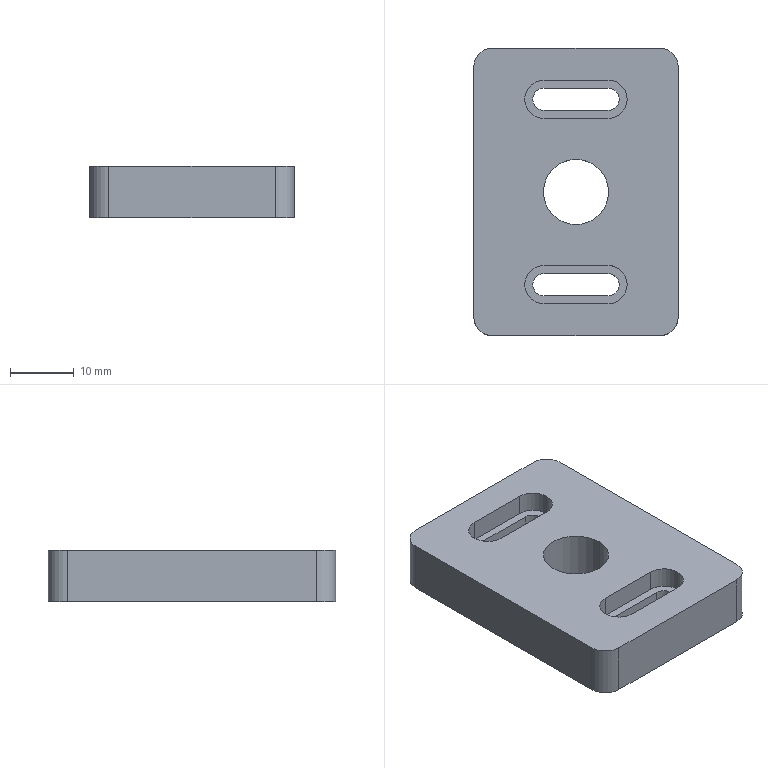Part | SolidWorks | features ICE 2, Extrusion 1, Fillet 1, HoleWzd 1 | 1 solid | 34 faces | box 32 x 45 x 8 mm | volume 9802 mm3 | cylinder 18 | plane 16 | commonest cylinder face diameters 6 x10 3.5 x6 10.2 x2
STEP:
#1=CARTESIAN_POINT('',(8.,14.5,4.7));
#2=VERTEX_POINT('',#1);
#3=CARTESIAN_POINT('',(5.,17.5,4.7));
#4=VERTEX_POINT('',#3);
#5=CARTESIAN_POINT('',(5.,14.5,4.7));
#6=DIRECTION('',(0.,0.,1.));
#7=DIRECTION('',(1.,0.,0.));
#8=AXIS2_PLACEMENT_3D('',#5,#6,#7);
#9=CIRCLE('',#8,3.);
#10=EDGE_CURVE('',#2,#4,#9,.T.);
#11=ORIENTED_EDGE('',*,*,#10,.F.);
#12=CARTESIAN_POINT('',(8.,14.5,8.));
#13=VERTEX_POINT('',#12);
#14=CARTESIAN_POINT('',(8.,14.5,4.7));
#15=DIRECTION('',(0.,0.,1.));
#16=VECTOR('',#15,1000.);
#17=LINE('',#14,#16);
#18=EDGE_CURVE('',#2,#13,#17,.T.);
#19=ORIENTED_EDGE('',*,*,#18,.T.);
#20=CARTESIAN_POINT('',(5.,17.5,8.));
#21=VERTEX_POINT('',#20);
#22=CARTESIAN_POINT('',(5.,14.5,8.));
#23=DIRECTION('',(0.,0.,1.));
#24=DIRECTION('',(1.,0.,0.));
#25=AXIS2_PLACEMENT_3D('',#22,#23,#24);
#26=CIRCLE('',#25,3.);
#27=EDGE_CURVE('',#13,#21,#26,.T.);
#28=ORIENTED_EDGE('',*,*,#27,.T.);
#29=CARTESIAN_POINT('',(5.,17.5,4.7));
#30=DIRECTION('',(0.,0.,1.));
#31=VECTOR('',#30,1000.);
#32=LINE('',#29,#31);
#33=EDGE_CURVE('',#4,#21,#32,.T.);
#34=ORIENTED_EDGE('',*,*,#33,.F.);
#35=EDGE_LOOP('',(#11,#19,#28,#34));
#36=FACE_OUTER_BOUND('',#35,.T.);
#37=CARTESIAN_POINT('',(5.,14.5,4.7));
#38=DIRECTION('',(0.,0.,1.));
#39=DIRECTION('',(1.,0.,0.));
#40=AXIS2_PLACEMENT_3D('',#37,#38,#39);
#41=CYLINDRICAL_SURFACE('',#40,3.);
#42=ADVANCED_FACE('',(#36),#41,.F.);
#43=CARTESIAN_POINT('',(8.,-14.5,4.7));
#44=VERTEX_POINT('',#43);
#45=CARTESIAN_POINT('',(5.,-11.5,4.7));
#46=VERTEX_POINT('',#45);
#47=CARTESIAN_POINT('',(5.,-14.5,4.7));
#48=DIRECTION('',(0.,0.,1.));
#49=DIRECTION('',(1.,0.,0.));
#50=AXIS2_PLACEMENT_3D('',#47,#48,#49);
#51=CIRCLE('',#50,3.);
#52=EDGE_CURVE('',#44,#46,#51,.T.);
#53=ORIENTED_EDGE('',*,*,#52,.F.);
#54=CARTESIAN_POINT('',(8.,-14.5,8.));
#55=VERTEX_POINT('',#54);
#56=CARTESIAN_POINT('',(8.,-14.5,4.7));
#57=DIRECTION('',(0.,0.,1.));
#58=VECTOR('',#57,1000.);
#59=LINE('',#56,#58);
#60=EDGE_CURVE('',#44,#55,#59,.T.);
#61=ORIENTED_EDGE('',*,*,#60,.T.);
#62=CARTESIAN_POINT('',(5.,-11.5,8.));
#63=VERTEX_POINT('',#62);
#64=CARTESIAN_POINT('',(5.,-14.5,8.));
#65=DIRECTION('',(0.,0.,1.));
#66=DIRECTION('',(1.,0.,0.));
#67=AXIS2_PLACEMENT_3D('',#64,#65,#66);
#68=CIRCLE('',#67,3.);
#69=EDGE_CURVE('',#55,#63,#68,.T.);
#70=ORIENTED_EDGE('',*,*,#69,.T.);
#71=CARTESIAN_POINT('',(5.,-11.5,4.7));
#72=DIRECTION('',(0.,0.,1.));
#73=VECTOR('',#72,1000.);
#74=LINE('',#71,#73);
#75=EDGE_CURVE('',#46,#63,#74,.T.);
#76=ORIENTED_EDGE('',*,*,#75,.F.);
#77=EDGE_LOOP('',(#53,#61,#70,#76));
#78=FACE_OUTER_BOUND('',#77,.T.);
#79=CARTESIAN_POINT('',(5.,-14.5,4.7));
#80=DIRECTION('',(0.,0.,1.));
#81=DIRECTION('',(1.,0.,0.));
#82=AXIS2_PLACEMENT_3D('',#79,#80,#81);
#83=CYLINDRICAL_SURFACE('',#82,3.);
#84=ADVANCED_FACE('',(#78),#83,.F.);
#85=CARTESIAN_POINT('',(-5.1,0.,0.));
#86=VERTEX_POINT('',#85);
#87=CARTESIAN_POINT('',(5.1,0.,0.));
#88=VERTEX_POINT('',#87);
#89=CARTESIAN_POINT('',(0.,0.,0.));
#90=DIRECTION('',(0.,0.,1.));
#91=DIRECTION('',(1.,0.,0.));
#92=AXIS2_PLACEMENT_3D('',#89,#90,#91);
#93=CIRCLE('',#92,5.1);
#94=EDGE_CURVE('',#86,#88,#93,.T.);
#95=ORIENTED_EDGE('',*,*,#94,.F.);
#96=CARTESIAN_POINT('',(-5.1,0.,8.));
#97=VERTEX_POINT('',#96);
#98=CARTESIAN_POINT('',(-5.1,0.,8.));
#99=DIRECTION('',(0.,0.,1.));
#100=VECTOR('',#99,1000.);
#101=LINE('',#98,#100);
#102=EDGE_CURVE('',#86,#97,#101,.T.);
#103=ORIENTED_EDGE('',*,*,#102,.T.);
#104=CARTESIAN_POINT('',(5.1,0.,8.));
#105=VERTEX_POINT('',#104);
#106=CARTESIAN_POINT('',(0.,0.,8.));
#107=DIRECTION('',(0.,0.,1.));
#108=DIRECTION('',(1.,0.,0.));
#109=AXIS2_PLACEMENT_3D('',#106,#107,#108);
#110=CIRCLE('',#109,5.1);
#111=EDGE_CURVE('',#97,#105,#110,.T.);
#112=ORIENTED_EDGE('',*,*,#111,.T.);
#113=CARTESIAN_POINT('',(5.1,0.,8.));
#114=DIRECTION('',(0.,0.,1.));
#115=VECTOR('',#114,1000.);
#116=LINE('',#113,#115);
#117=EDGE_CURVE('',#88,#105,#116,.T.);
#118=ORIENTED_EDGE('',*,*,#117,.F.);
#119=EDGE_LOOP('',(#95,#103,#112,#118));
#120=FACE_OUTER_BOUND('',#119,.T.);
#121=CARTESIAN_POINT('',(0.,0.,8.));
#122=DIRECTION('',(0.,0.,1.));
#123=DIRECTION('',(1.,0.,0.));
#124=AXIS2_PLACEMENT_3D('',#121,#122,#123);
#125=CYLINDRICAL_SURFACE('',#124,5.1);
#126=ADVANCED_FACE('',(#120),#125,.F.);
#127=CARTESIAN_POINT('',(6.75,-14.5,0.));
#128=VERTEX_POINT('',#127);
#129=CARTESIAN_POINT('',(5.,-12.75,0.));
#130=VERTEX_POINT('',#129);
#131=CARTESIAN_POINT('',(5.,-14.5,0.));
#132=DIRECTION('',(0.,0.,1.));
#133=DIRECTION('',(1.,0.,0.));
#134=AXIS2_PLACEMENT_3D('',#131,#132,#133);
#135=CIRCLE('',#134,1.75);
#136=EDGE_CURVE('',#128,#130,#135,.T.);
#137=ORIENTED_EDGE('',*,*,#136,.F.);
#138=CARTESIAN_POINT('',(6.75,-14.5,4.7));
#139=VERTEX_POINT('',#138);
#140=CARTESIAN_POINT('',(6.75,-14.5,0.));
#141=DIRECTION('',(0.,0.,1.));
#142=VECTOR('',#141,1000.);
#143=LINE('',#140,#142);
#144=EDGE_CURVE('',#128,#139,#143,.T.);
#145=ORIENTED_EDGE('',*,*,#144,.T.);
#146=CARTESIAN_POINT('',(5.,-12.75,4.7));
#147=VERTEX_POINT('',#146);
#148=CARTESIAN_POINT('',(5.,-14.5,4.7));
#149=DIRECTION('',(0.,0.,-1.));
#150=DIRECTION('',(1.,0.,0.));
#151=AXIS2_PLACEMENT_3D('',#148,#149,#150);
#152=CIRCLE('',#151,1.75);
#153=EDGE_CURVE('',#147,#139,#152,.T.);
#154=ORIENTED_EDGE('',*,*,#153,.F.);
#155=CARTESIAN_POINT('',(5.,-12.75,0.));
#156=DIRECTION('',(0.,0.,1.));
#157=VECTOR('',#156,1000.);
#158=LINE('',#155,#157);
#159=EDGE_CURVE('',#130,#147,#158,.T.);
#160=ORIENTED_EDGE('',*,*,#159,.F.);
#161=EDGE_LOOP('',(#137,#145,#154,#160));
#162=FACE_OUTER_BOUND('',#161,.T.);
#163=CARTESIAN_POINT('',(5.,-14.5,0.));
#164=DIRECTION('',(0.,0.,1.));
#165=DIRECTION('',(1.,0.,0.));
#166=AXIS2_PLACEMENT_3D('',#163,#164,#165);
#167=CYLINDRICAL_SURFACE('',#166,1.75);
#168=ADVANCED_FACE('',(#162),#167,.F.);
#169=CARTESIAN_POINT('',(6.75,14.5,0.));
#170=VERTEX_POINT('',#169);
#171=CARTESIAN_POINT('',(5.,16.25,0.));
#172=VERTEX_POINT('',#171);
#173=CARTESIAN_POINT('',(5.,14.5,0.));
#174=DIRECTION('',(0.,0.,1.));
#175=DIRECTION('',(1.,0.,0.));
#176=AXIS2_PLACEMENT_3D('',#173,#174,#175);
#177=CIRCLE('',#176,1.75);
#178=EDGE_CURVE('',#170,#172,#177,.T.);
#179=ORIENTED_EDGE('',*,*,#178,.F.);
#180=CARTESIAN_POINT('',(6.75,14.5,4.7));
#181=VERTEX_POINT('',#180);
#182=CARTESIAN_POINT('',(6.75,14.5,0.));
#183=DIRECTION('',(0.,0.,1.));
#184=VECTOR('',#183,1000.);
#185=LINE('',#182,#184);
#186=EDGE_CURVE('',#170,#181,#185,.T.);
#187=ORIENTED_EDGE('',*,*,#186,.T.);
#188=CARTESIAN_POINT('',(5.,16.25,4.7));
#189=VERTEX_POINT('',#188);
#190=CARTESIAN_POINT('',(5.,14.5,4.7));
#191=DIRECTION('',(0.,0.,-1.));
#192=DIRECTION('',(1.,0.,0.));
#193=AXIS2_PLACEMENT_3D('',#190,#191,#192);
#194=CIRCLE('',#193,1.75);
#195=EDGE_CURVE('',#189,#181,#194,.T.);
#196=ORIENTED_EDGE('',*,*,#195,.F.);
#197=CARTESIAN_POINT('',(5.,16.25,0.));
#198=DIRECTION('',(0.,0.,1.));
#199=VECTOR('',#198,1000.);
#200=LINE('',#197,#199);
#201=EDGE_CURVE('',#172,#189,#200,.T.);
#202=ORIENTED_EDGE('',*,*,#201,.F.);
#203=EDGE_LOOP('',(#179,#187,#196,#202));
#204=FACE_OUTER_BOUND('',#203,.T.);
#205=CARTESIAN_POINT('',(5.,14.5,0.));
#206=DIRECTION('',(0.,0.,1.));
#207=DIRECTION('',(1.,0.,0.));
#208=AXIS2_PLACEMENT_3D('',#205,#206,#207);
#209=CYLINDRICAL_SURFACE('',#208,1.75);
#210=ADVANCED_FACE('',(#204),#209,.F.);
#211=CARTESIAN_POINT('',(-5.,12.75,4.7));
#212=VERTEX_POINT('',#211);
#213=CARTESIAN_POINT('',(-5.,16.25,4.7));
#214=VERTEX_POINT('',#213);
#215=CARTESIAN_POINT('',(-5.,14.5,4.7));
#216=DIRECTION('',(0.,0.,-1.));
#217=DIRECTION('',(1.,0.,0.));
#218=AXIS2_PLACEMENT_3D('',#215,#216,#217);
#219=CIRCLE('',#218,1.75);
#220=EDGE_CURVE('',#212,#214,#219,.T.);
#221=ORIENTED_EDGE('',*,*,#220,.F.);
#222=CARTESIAN_POINT('',(-5.,12.75,0.));
#223=VERTEX_POINT('',#222);
#224=CARTESIAN_POINT('',(-5.,12.75,0.));
#225=DIRECTION('',(0.,0.,1.));
#226=VECTOR('',#225,1000.);
#227=LINE('',#224,#226);
#228=EDGE_CURVE('',#223,#212,#227,.T.);
#229=ORIENTED_EDGE('',*,*,#228,.F.);
#230=CARTESIAN_POINT('',(-5.,16.25,0.));
#231=VERTEX_POINT('',#230);
#232=CARTESIAN_POINT('',(-5.,14.5,0.));
#233=DIRECTION('',(0.,0.,1.));
#234=DIRECTION('',(1.,0.,0.));
#235=AXIS2_PLACEMENT_3D('',#232,#233,#234);
#236=CIRCLE('',#235,1.75);
#237=EDGE_CURVE('',#231,#223,#236,.T.);
#238=ORIENTED_EDGE('',*,*,#237,.F.);
#239=CARTESIAN_POINT('',(-5.,16.25,0.));
#240=DIRECTION('',(0.,0.,1.));
#241=VECTOR('',#240,1000.);
#242=LINE('',#239,#241);
#243=EDGE_CURVE('',#231,#214,#242,.T.);
#244=ORIENTED_EDGE('',*,*,#243,.T.);
#245=EDGE_LOOP('',(#221,#229,#238,#244));
#246=FACE_OUTER_BOUND('',#245,.T.);
#247=CARTESIAN_POINT('',(-5.,14.5,0.));
#248=DIRECTION('',(0.,0.,1.));
#249=DIRECTION('',(1.,0.,0.));
#250=AXIS2_PLACEMENT_3D('',#247,#248,#249);
#251=CYLINDRICAL_SURFACE('',#250,1.75);
#252=ADVANCED_FACE('',(#246),#251,.F.);
#253=CARTESIAN_POINT('',(-5.,16.25,4.7));
#254=DIRECTION('',(1.,0.,0.));
#255=VECTOR('',#254,1000.);
#256=LINE('',#253,#255);
#257=EDGE_CURVE('',#214,#189,#256,.T.);
#258=ORIENTED_EDGE('',*,*,#257,.F.);
#259=ORIENTED_EDGE('',*,*,#243,.F.);
#260=CARTESIAN_POINT('',(-5.,16.25,0.));
#261=DIRECTION('',(-1.,0.,0.));
#262=VECTOR('',#261,1000.);
#263=LINE('',#260,#262);
#264=EDGE_CURVE('',#172,#231,#263,.T.);
#265=ORIENTED_EDGE('',*,*,#264,.F.);
#266=ORIENTED_EDGE('',*,*,#201,.T.);
#267=EDGE_LOOP('',(#258,#259,#265,#266));
#268=FACE_OUTER_BOUND('',#267,.T.);
#269=CARTESIAN_POINT('',(-5.,16.25,0.));
#270=DIRECTION('',(0.,1.,0.));
#271=DIRECTION('',(-1.,0.,0.));
#272=AXIS2_PLACEMENT_3D('',#269,#270,#271);
#273=PLANE('',#272);
#274=ADVANCED_FACE('',(#268),#273,.F.);
#275=ORIENTED_EDGE('',*,*,#186,.F.);
#276=CARTESIAN_POINT('',(5.,12.75,0.));
#277=VERTEX_POINT('',#276);
#278=CARTESIAN_POINT('',(5.,14.5,0.));
#279=DIRECTION('',(0.,0.,1.));
#280=DIRECTION('',(1.,0.,0.));
#281=AXIS2_PLACEMENT_3D('',#278,#279,#280);
#282=CIRCLE('',#281,1.75);
#283=EDGE_CURVE('',#277,#170,#282,.T.);
#284=ORIENTED_EDGE('',*,*,#283,.F.);
#285=CARTESIAN_POINT('',(5.,12.75,4.7));
#286=VERTEX_POINT('',#285);
#287=CARTESIAN_POINT('',(5.,12.75,0.));
#288=DIRECTION('',(0.,0.,1.));
#289=VECTOR('',#288,1000.);
#290=LINE('',#287,#289);
#291=EDGE_CURVE('',#277,#286,#290,.T.);
#292=ORIENTED_EDGE('',*,*,#291,.T.);
#293=CARTESIAN_POINT('',(5.,14.5,4.7));
#294=DIRECTION('',(0.,0.,-1.));
#295=DIRECTION('',(1.,0.,0.));
#296=AXIS2_PLACEMENT_3D('',#293,#294,#295);
#297=CIRCLE('',#296,1.75);
#298=EDGE_CURVE('',#181,#286,#297,.T.);
#299=ORIENTED_EDGE('',*,*,#298,.F.);
#300=EDGE_LOOP('',(#275,#284,#292,#299));
#301=FACE_OUTER_BOUND('',#300,.T.);
#302=CARTESIAN_POINT('',(5.,14.5,0.));
#303=DIRECTION('',(0.,0.,1.));
#304=DIRECTION('',(1.,0.,0.));
#305=AXIS2_PLACEMENT_3D('',#302,#303,#304);
#306=CYLINDRICAL_SURFACE('',#305,1.75);
#307=ADVANCED_FACE('',(#301),#306,.F.);
#308=CARTESIAN_POINT('',(-5.,12.75,4.7));
#309=DIRECTION('',(-1.,0.,0.));
#310=VECTOR('',#309,1000.);
#311=LINE('',#308,#310);
#312=EDGE_CURVE('',#286,#212,#311,.T.);
#313=ORIENTED_EDGE('',*,*,#312,.F.);
#314=ORIENTED_EDGE('',*,*,#291,.F.);
#315=CARTESIAN_POINT('',(-5.,12.75,0.));
#316=DIRECTION('',(1.,0.,0.));
#317=VECTOR('',#316,1000.);
#318=LINE('',#315,#317);
#319=EDGE_CURVE('',#223,#277,#318,.T.);
#320=ORIENTED_EDGE('',*,*,#319,.F.);
#321=ORIENTED_EDGE('',*,*,#228,.T.);
#322=EDGE_LOOP('',(#313,#314,#320,#321));
#323=FACE_OUTER_BOUND('',#322,.T.);
#324=CARTESIAN_POINT('',(-5.,12.75,0.));
#325=DIRECTION('',(0.,-1.,0.));
#326=DIRECTION('',(0.,0.,-1.));
#327=AXIS2_PLACEMENT_3D('',#324,#325,#326);
#328=PLANE('',#327);
#329=ADVANCED_FACE('',(#323),#328,.F.);
#330=CARTESIAN_POINT('',(-5.,-16.25,4.7));
#331=VERTEX_POINT('',#330);
#332=CARTESIAN_POINT('',(-5.,-12.75,4.7));
#333=VERTEX_POINT('',#332);
#334=CARTESIAN_POINT('',(-5.,-14.5,4.7));
#335=DIRECTION('',(0.,0.,-1.));
#336=DIRECTION('',(1.,0.,0.));
#337=AXIS2_PLACEMENT_3D('',#334,#335,#336);
#338=CIRCLE('',#337,1.75);
#339=EDGE_CURVE('',#331,#333,#338,.T.);
#340=ORIENTED_EDGE('',*,*,#339,.F.);
#341=CARTESIAN_POINT('',(-5.,-16.25,0.));
#342=VERTEX_POINT('',#341);
#343=CARTESIAN_POINT('',(-5.,-16.25,0.));
#344=DIRECTION('',(0.,0.,1.));
#345=VECTOR('',#344,1000.);
#346=LINE('',#343,#345);
#347=EDGE_CURVE('',#342,#331,#346,.T.);
#348=ORIENTED_EDGE('',*,*,#347,.F.);
#349=CARTESIAN_POINT('',(-5.,-12.75,0.));
#350=VERTEX_POINT('',#349);
#351=CARTESIAN_POINT('',(-5.,-14.5,0.));
#352=DIRECTION('',(0.,0.,1.));
#353=DIRECTION('',(1.,0.,0.));
#354=AXIS2_PLACEMENT_3D('',#351,#352,#353);
#355=CIRCLE('',#354,1.75);
#356=EDGE_CURVE('',#350,#342,#355,.T.);
#357=ORIENTED_EDGE('',*,*,#356,.F.);
#358=CARTESIAN_POINT('',(-5.,-12.75,0.));
#359=DIRECTION('',(0.,0.,1.));
#360=VECTOR('',#359,1000.);
#361=LINE('',#358,#360);
#362=EDGE_CURVE('',#350,#333,#361,.T.);
#363=ORIENTED_EDGE('',*,*,#362,.T.);
#364=EDGE_LOOP('',(#340,#348,#357,#363));
#365=FACE_OUTER_BOUND('',#364,.T.);
#366=CARTESIAN_POINT('',(-5.,-14.5,0.));
#367=DIRECTION('',(0.,0.,1.));
#368=DIRECTION('',(1.,0.,0.));
#369=AXIS2_PLACEMENT_3D('',#366,#367,#368);
#370=CYLINDRICAL_SURFACE('',#369,1.75);
#371=ADVANCED_FACE('',(#365),#370,.F.);
#372=CARTESIAN_POINT('',(-5.,-12.75,4.7));
#373=DIRECTION('',(1.,0.,0.));
#374=VECTOR('',#373,1000.);
#375=LINE('',#372,#374);
#376=EDGE_CURVE('',#333,#147,#375,.T.);
#377=ORIENTED_EDGE('',*,*,#376,.F.);
#378=ORIENTED_EDGE('',*,*,#362,.F.);
#379=CARTESIAN_POINT('',(-5.,-12.75,0.));
#380=DIRECTION('',(-1.,0.,0.));
#381=VECTOR('',#380,1000.);
#382=LINE('',#379,#381);
#383=EDGE_CURVE('',#130,#350,#382,.T.);
#384=ORIENTED_EDGE('',*,*,#383,.F.);
#385=ORIENTED_EDGE('',*,*,#159,.T.);
#386=EDGE_LOOP('',(#377,#378,#384,#385));
#387=FACE_OUTER_BOUND('',#386,.T.);
#388=CARTESIAN_POINT('',(-5.,-12.75,0.));
#389=DIRECTION('',(0.,1.,0.));
#390=DIRECTION('',(0.,0.,1.));
#391=AXIS2_PLACEMENT_3D('',#388,#389,#390);
#392=PLANE('',#391);
#393=ADVANCED_FACE('',(#387),#392,.F.);
#394=ORIENTED_EDGE('',*,*,#144,.F.);
#395=CARTESIAN_POINT('',(5.,-16.25,0.));
#396=VERTEX_POINT('',#395);
#397=CARTESIAN_POINT('',(5.,-14.5,0.));
#398=DIRECTION('',(0.,0.,1.));
#399=DIRECTION('',(1.,0.,0.));
#400=AXIS2_PLACEMENT_3D('',#397,#398,#399);
#401=CIRCLE('',#400,1.75);
#402=EDGE_CURVE('',#396,#128,#401,.T.);
#403=ORIENTED_EDGE('',*,*,#402,.F.);
#404=CARTESIAN_POINT('',(5.,-16.25,4.7));
#405=VERTEX_POINT('',#404);
#406=CARTESIAN_POINT('',(5.,-16.25,0.));
#407=DIRECTION('',(0.,0.,1.));
#408=VECTOR('',#407,1000.);
#409=LINE('',#406,#408);
#410=EDGE_CURVE('',#396,#405,#409,.T.);
#411=ORIENTED_EDGE('',*,*,#410,.T.);
#412=CARTESIAN_POINT('',(5.,-14.5,4.7));
#413=DIRECTION('',(0.,0.,-1.));
#414=DIRECTION('',(1.,0.,0.));
#415=AXIS2_PLACEMENT_3D('',#412,#413,#414);
#416=CIRCLE('',#415,1.75);
#417=EDGE_CURVE('',#139,#405,#416,.T.);
#418=ORIENTED_EDGE('',*,*,#417,.F.);
#419=EDGE_LOOP('',(#394,#403,#411,#418));
#420=FACE_OUTER_BOUND('',#419,.T.);
#421=CARTESIAN_POINT('',(5.,-14.5,0.));
#422=DIRECTION('',(0.,0.,1.));
#423=DIRECTION('',(1.,0.,0.));
#424=AXIS2_PLACEMENT_3D('',#421,#422,#423);
#425=CYLINDRICAL_SURFACE('',#424,1.75);
#426=ADVANCED_FACE('',(#420),#425,.F.);
#427=CARTESIAN_POINT('',(-5.,-16.25,4.7));
#428=DIRECTION('',(-1.,0.,0.));
#429=VECTOR('',#428,1000.);
#430=LINE('',#427,#429);
#431=EDGE_CURVE('',#405,#331,#430,.T.);
#432=ORIENTED_EDGE('',*,*,#431,.F.);
#433=ORIENTED_EDGE('',*,*,#410,.F.);
#434=CARTESIAN_POINT('',(-5.,-16.25,0.));
#435=DIRECTION('',(1.,0.,0.));
#436=VECTOR('',#435,1000.);
#437=LINE('',#434,#436);
#438=EDGE_CURVE('',#342,#396,#437,.T.);
#439=ORIENTED_EDGE('',*,*,#438,.F.);
#440=ORIENTED_EDGE('',*,*,#347,.T.);
#441=EDGE_LOOP('',(#432,#433,#439,#440));
#442=FACE_OUTER_BOUND('',#441,.T.);
#443=CARTESIAN_POINT('',(-5.,-16.25,0.));
#444=DIRECTION('',(0.,-1.,0.));
#445=DIRECTION('',(1.,0.,0.));
#446=AXIS2_PLACEMENT_3D('',#443,#444,#445);
#447=PLANE('',#446);
#448=ADVANCED_FACE('',(#442),#447,.F.);
#449=CARTESIAN_POINT('',(-16.,19.5,8.));
#450=VERTEX_POINT('',#449);
#451=CARTESIAN_POINT('',(-16.,-19.5,8.));
#452=VERTEX_POINT('',#451);
#453=CARTESIAN_POINT('',(-16.,-22.5,8.));
#454=DIRECTION('',(0.,-1.,0.));
#455=VECTOR('',#454,1000.);
#456=LINE('',#453,#455);
#457=EDGE_CURVE('',#450,#452,#456,.T.);
#458=ORIENTED_EDGE('',*,*,#457,.F.);
#459=CARTESIAN_POINT('',(-16.,19.5,0.));
#460=VERTEX_POINT('',#459);
#461=CARTESIAN_POINT('',(-16.,19.5,8.));
#462=DIRECTION('',(0.,0.,-1.));
#463=VECTOR('',#462,1000.);
#464=LINE('',#461,#463);
#465=EDGE_CURVE('',#450,#460,#464,.T.);
#466=ORIENTED_EDGE('',*,*,#465,.T.);
#467=CARTESIAN_POINT('',(-16.,-19.5,0.));
#468=VERTEX_POINT('',#467);
#469=CARTESIAN_POINT('',(-16.,-22.5,0.));
#470=DIRECTION('',(0.,-1.,0.));
#471=VECTOR('',#470,1000.);
#472=LINE('',#469,#471);
#473=EDGE_CURVE('',#460,#468,#472,.T.);
#474=ORIENTED_EDGE('',*,*,#473,.T.);
#475=CARTESIAN_POINT('',(-16.,-19.5,8.));
#476=DIRECTION('',(0.,0.,1.));
#477=VECTOR('',#476,1000.);
#478=LINE('',#475,#477);
#479=EDGE_CURVE('',#468,#452,#478,.T.);
#480=ORIENTED_EDGE('',*,*,#479,.T.);
#481=EDGE_LOOP('',(#458,#466,#474,#480));
#482=FACE_OUTER_BOUND('',#481,.T.);
#483=CARTESIAN_POINT('',(-16.,-22.5,8.));
#484=DIRECTION('',(1.,0.,0.));
#485=DIRECTION('',(0.,0.,-1.));
#486=AXIS2_PLACEMENT_3D('',#483,#484,#485);
#487=PLANE('',#486);
#488=ADVANCED_FACE('',(#482),#487,.F.);
#489=CARTESIAN_POINT('',(-13.,-22.5,0.));
#490=VERTEX_POINT('',#489);
#491=CARTESIAN_POINT('',(13.,-22.5,0.));
#492=VERTEX_POINT('',#491);
#493=CARTESIAN_POINT('',(16.,-22.5,0.));
#494=DIRECTION('',(1.,0.,0.));
#495=VECTOR('',#494,1000.);
#496=LINE('',#493,#495);
#497=EDGE_CURVE('',#490,#492,#496,.T.);
#498=ORIENTED_EDGE('',*,*,#497,.T.);
#499=CARTESIAN_POINT('',(13.,-22.5,8.));
#500=VERTEX_POINT('',#499);
#501=CARTESIAN_POINT('',(13.,-22.5,8.));
#502=DIRECTION('',(0.,0.,1.));
#503=VECTOR('',#502,1000.);
#504=LINE('',#501,#503);
#505=EDGE_CURVE('',#492,#500,#504,.T.);
#506=ORIENTED_EDGE('',*,*,#505,.T.);
#507=CARTESIAN_POINT('',(-13.,-22.5,8.));
#508=VERTEX_POINT('',#507);
#509=CARTESIAN_POINT('',(16.,-22.5,8.));
#510=DIRECTION('',(1.,0.,0.));
#511=VECTOR('',#510,1000.);
#512=LINE('',#509,#511);
#513=EDGE_CURVE('',#508,#500,#512,.T.);
#514=ORIENTED_EDGE('',*,*,#513,.F.);
#515=CARTESIAN_POINT('',(-13.,-22.5,8.));
#516=DIRECTION('',(0.,0.,-1.));
#517=VECTOR('',#516,1000.);
#518=LINE('',#515,#517);
#519=EDGE_CURVE('',#508,#490,#518,.T.);
#520=ORIENTED_EDGE('',*,*,#519,.T.);
#521=EDGE_LOOP('',(#498,#506,#514,#520));
#522=FACE_OUTER_BOUND('',#521,.T.);
#523=CARTESIAN_POINT('',(16.,-22.5,8.));
#524=DIRECTION('',(0.,1.,0.));
#525=DIRECTION('',(-1.,0.,0.));
#526=AXIS2_PLACEMENT_3D('',#523,#524,#525);
#527=PLANE('',#526);
#528=ADVANCED_FACE('',(#522),#527,.F.);
#529=CARTESIAN_POINT('',(16.,-19.5,0.));
#530=VERTEX_POINT('',#529);
#531=CARTESIAN_POINT('',(16.,19.5,0.));
#532=VERTEX_POINT('',#531);
#533=CARTESIAN_POINT('',(16.,-22.5,0.));
#534=DIRECTION('',(0.,1.,0.));
#535=VECTOR('',#534,1000.);
#536=LINE('',#533,#535);
#537=EDGE_CURVE('',#530,#532,#536,.T.);
#538=ORIENTED_EDGE('',*,*,#537,.T.);
#539=CARTESIAN_POINT('',(16.,19.5,8.));
#540=VERTEX_POINT('',#539);
#541=CARTESIAN_POINT('',(16.,19.5,8.));
#542=DIRECTION('',(0.,0.,1.));
#543=VECTOR('',#542,1000.);
#544=LINE('',#541,#543);
#545=EDGE_CURVE('',#532,#540,#544,.T.);
#546=ORIENTED_EDGE('',*,*,#545,.T.);
#547=CARTESIAN_POINT('',(16.,-19.5,8.));
#548=VERTEX_POINT('',#547);
#549=CARTESIAN_POINT('',(16.,-22.5,8.));
#550=DIRECTION('',(0.,1.,0.));
#551=VECTOR('',#550,1000.);
#552=LINE('',#549,#551);
#553=EDGE_CURVE('',#548,#540,#552,.T.);
#554=ORIENTED_EDGE('',*,*,#553,.F.);
#555=CARTESIAN_POINT('',(16.,-19.5,8.));
#556=DIRECTION('',(0.,0.,-1.));
#557=VECTOR('',#556,1000.);
#558=LINE('',#555,#557);
#559=EDGE_CURVE('',#548,#530,#558,.T.);
#560=ORIENTED_EDGE('',*,*,#559,.T.);
#561=EDGE_LOOP('',(#538,#546,#554,#560));
#562=FACE_OUTER_BOUND('',#561,.T.);
#563=CARTESIAN_POINT('',(16.,-22.5,8.));
#564=DIRECTION('',(-1.,0.,0.));
#565=DIRECTION('',(0.,0.,1.));
#566=AXIS2_PLACEMENT_3D('',#563,#564,#565);
#567=PLANE('',#566);
#568=ADVANCED_FACE('',(#562),#567,.F.);
#569=CARTESIAN_POINT('',(13.,22.5,0.));
#570=VERTEX_POINT('',#569);
#571=CARTESIAN_POINT('',(-13.,22.5,0.));
#572=VERTEX_POINT('',#571);
#573=CARTESIAN_POINT('',(16.,22.5,0.));
#574=DIRECTION('',(-1.,0.,0.));
#575=VECTOR('',#574,1000.);
#576=LINE('',#573,#575);
#577=EDGE_CURVE('',#570,#572,#576,.T.);
#578=ORIENTED_EDGE('',*,*,#577,.T.);
#579=CARTESIAN_POINT('',(-13.,22.5,8.));
#580=VERTEX_POINT('',#579);
#581=CARTESIAN_POINT('',(-13.,22.5,8.));
#582=DIRECTION('',(0.,0.,1.));
#583=VECTOR('',#582,1000.);
#584=LINE('',#581,#583);
#585=EDGE_CURVE('',#572,#580,#584,.T.);
#586=ORIENTED_EDGE('',*,*,#585,.T.);
#587=CARTESIAN_POINT('',(13.,22.5,8.));
#588=VERTEX_POINT('',#587);
#589=CARTESIAN_POINT('',(16.,22.5,8.));
#590=DIRECTION('',(-1.,0.,0.));
#591=VECTOR('',#590,1000.);
#592=LINE('',#589,#591);
#593=EDGE_CURVE('',#588,#580,#592,.T.);
#594=ORIENTED_EDGE('',*,*,#593,.F.);
#595=CARTESIAN_POINT('',(13.,22.5,8.));
#596=DIRECTION('',(0.,0.,-1.));
#597=VECTOR('',#596,1000.);
#598=LINE('',#595,#597);
#599=EDGE_CURVE('',#588,#570,#598,.T.);
#600=ORIENTED_EDGE('',*,*,#599,.T.);
#601=EDGE_LOOP('',(#578,#586,#594,#600));
#602=FACE_OUTER_BOUND('',#601,.T.);
#603=CARTESIAN_POINT('',(16.,22.5,8.));
#604=DIRECTION('',(0.,-1.,0.));
#605=DIRECTION('',(1.,0.,0.));
#606=AXIS2_PLACEMENT_3D('',#603,#604,#605);
#607=PLANE('',#606);
#608=ADVANCED_FACE('',(#602),#607,.F.);
#609=CARTESIAN_POINT('',(-5.,-11.5,8.));
#610=VERTEX_POINT('',#609);
#611=CARTESIAN_POINT('',(-5.,-17.5,8.));
#612=VERTEX_POINT('',#611);
#613=CARTESIAN_POINT('',(-5.,-14.5,8.));
#614=DIRECTION('',(0.,0.,1.));
#615=DIRECTION('',(1.,0.,0.));
#616=AXIS2_PLACEMENT_3D('',#613,#614,#615);
#617=CIRCLE('',#616,3.);
#618=EDGE_CURVE('',#610,#612,#617,.T.);
#619=ORIENTED_EDGE('',*,*,#618,.F.);
#620=CARTESIAN_POINT('',(-5.,-11.5,8.));
#621=DIRECTION('',(-1.,0.,0.));
#622=VECTOR('',#621,1000.);
#623=LINE('',#620,#622);
#624=EDGE_CURVE('',#63,#610,#623,.T.);
#625=ORIENTED_EDGE('',*,*,#624,.F.);
#626=ORIENTED_EDGE('',*,*,#69,.F.);
#627=CARTESIAN_POINT('',(5.,-17.5,8.));
#628=VERTEX_POINT('',#627);
#629=CARTESIAN_POINT('',(5.,-14.5,8.));
#630=DIRECTION('',(0.,0.,1.));
#631=DIRECTION('',(1.,0.,0.));
#632=AXIS2_PLACEMENT_3D('',#629,#630,#631);
#633=CIRCLE('',#632,3.);
#634=EDGE_CURVE('',#628,#55,#633,.T.);
#635=ORIENTED_EDGE('',*,*,#634,.F.);
#636=CARTESIAN_POINT('',(-5.,-17.5,8.));
#637=DIRECTION('',(1.,0.,0.));
#638=VECTOR('',#637,1000.);
#639=LINE('',#636,#638);
#640=EDGE_CURVE('',#612,#628,#639,.T.);
#641=ORIENTED_EDGE('',*,*,#640,.F.);
#642=EDGE_LOOP('',(#619,#625,#626,#635,#641));
#643=FACE_BOUND('',#642,.T.);
#644=CARTESIAN_POINT('',(-5.,17.5,8.));
#645=VERTEX_POINT('',#644);
#646=CARTESIAN_POINT('',(-5.,11.5,8.));
#647=VERTEX_POINT('',#646);
#648=CARTESIAN_POINT('',(-5.,14.5,8.));
#649=DIRECTION('',(0.,0.,1.));
#650=DIRECTION('',(1.,0.,0.));
#651=AXIS2_PLACEMENT_3D('',#648,#649,#650);
#652=CIRCLE('',#651,3.);
#653=EDGE_CURVE('',#645,#647,#652,.T.);
#654=ORIENTED_EDGE('',*,*,#653,.F.);
#655=CARTESIAN_POINT('',(-5.,17.5,8.));
#656=DIRECTION('',(-1.,0.,0.));
#657=VECTOR('',#656,1000.);
#658=LINE('',#655,#657);
#659=EDGE_CURVE('',#21,#645,#658,.T.);
#660=ORIENTED_EDGE('',*,*,#659,.F.);
#661=ORIENTED_EDGE('',*,*,#27,.F.);
#662=CARTESIAN_POINT('',(5.,11.5,8.));
#663=VERTEX_POINT('',#662);
#664=CARTESIAN_POINT('',(5.,14.5,8.));
#665=DIRECTION('',(0.,0.,1.));
#666=DIRECTION('',(1.,0.,0.));
#667=AXIS2_PLACEMENT_3D('',#664,#665,#666);
#668=CIRCLE('',#667,3.);
#669=EDGE_CURVE('',#663,#13,#668,.T.);
#670=ORIENTED_EDGE('',*,*,#669,.F.);
#671=CARTESIAN_POINT('',(-5.,11.5,8.));
#672=DIRECTION('',(1.,0.,0.));
#673=VECTOR('',#672,1000.);
#674=LINE('',#671,#673);
#675=EDGE_CURVE('',#647,#663,#674,.T.);
#676=ORIENTED_EDGE('',*,*,#675,.F.);
#677=EDGE_LOOP('',(#654,#660,#661,#670,#676));
#678=FACE_BOUND('',#677,.T.);
#679=CARTESIAN_POINT('',(0.,0.,8.));
#680=DIRECTION('',(0.,0.,1.));
#681=DIRECTION('',(1.,0.,0.));
#682=AXIS2_PLACEMENT_3D('',#679,#680,#681);
#683=CIRCLE('',#682,5.1);
#684=EDGE_CURVE('',#105,#97,#683,.T.);
#685=ORIENTED_EDGE('',*,*,#684,.F.);
#686=ORIENTED_EDGE('',*,*,#111,.F.);
#687=EDGE_LOOP('',(#685,#686));
#688=FACE_BOUND('',#687,.T.);
#689=ORIENTED_EDGE('',*,*,#593,.T.);
#690=CARTESIAN_POINT('',(-13.,19.5,8.));
#691=DIRECTION('',(0.,0.,1.));
#692=DIRECTION('',(1.,0.,0.));
#693=AXIS2_PLACEMENT_3D('',#690,#691,#692);
#694=CIRCLE('',#693,3.);
#695=EDGE_CURVE('',#580,#450,#694,.T.);
#696=ORIENTED_EDGE('',*,*,#695,.T.);
#697=ORIENTED_EDGE('',*,*,#457,.T.);
#698=CARTESIAN_POINT('',(-13.,-19.5,8.));
#699=DIRECTION('',(0.,0.,1.));
#700=DIRECTION('',(1.,0.,0.));
#701=AXIS2_PLACEMENT_3D('',#698,#699,#700);
#702=CIRCLE('',#701,3.);
#703=EDGE_CURVE('',#452,#508,#702,.T.);
#704=ORIENTED_EDGE('',*,*,#703,.T.);
#705=ORIENTED_EDGE('',*,*,#513,.T.);
#706=CARTESIAN_POINT('',(13.,-19.5,8.));
#707=DIRECTION('',(0.,0.,1.));
#708=DIRECTION('',(1.,0.,0.));
#709=AXIS2_PLACEMENT_3D('',#706,#707,#708);
#710=CIRCLE('',#709,3.);
#711=EDGE_CURVE('',#500,#548,#710,.T.);
#712=ORIENTED_EDGE('',*,*,#711,.T.);
#713=ORIENTED_EDGE('',*,*,#553,.T.);
#714=CARTESIAN_POINT('',(13.,19.5,8.));
#715=DIRECTION('',(0.,0.,1.));
#716=DIRECTION('',(1.,0.,0.));
#717=AXIS2_PLACEMENT_3D('',#714,#715,#716);
#718=CIRCLE('',#717,3.);
#719=EDGE_CURVE('',#540,#588,#718,.T.);
#720=ORIENTED_EDGE('',*,*,#719,.T.);
#721=EDGE_LOOP('',(#689,#696,#697,#704,#705,#712,#713,#720));
#722=FACE_OUTER_BOUND('',#721,.T.);
#723=CARTESIAN_POINT('',(0.,0.,8.));
#724=DIRECTION('',(0.,0.,1.));
#725=DIRECTION('',(1.,0.,0.));
#726=AXIS2_PLACEMENT_3D('',#723,#724,#725);
#727=PLANE('',#726);
#728=ADVANCED_FACE('',(#643,#678,#688,#722),#727,.T.);
#729=ORIENTED_EDGE('',*,*,#383,.T.);
#730=ORIENTED_EDGE('',*,*,#356,.T.);
#731=ORIENTED_EDGE('',*,*,#438,.T.);
#732=ORIENTED_EDGE('',*,*,#402,.T.);
#733=ORIENTED_EDGE('',*,*,#136,.T.);
#734=EDGE_LOOP('',(#729,#730,#731,#732,#733));
#735=FACE_BOUND('',#734,.T.);
#736=ORIENTED_EDGE('',*,*,#264,.T.);
#737=ORIENTED_EDGE('',*,*,#237,.T.);
#738=ORIENTED_EDGE('',*,*,#319,.T.);
#739=ORIENTED_EDGE('',*,*,#283,.T.);
#740=ORIENTED_EDGE('',*,*,#178,.T.);
#741=EDGE_LOOP('',(#736,#737,#738,#739,#740));
#742=FACE_BOUND('',#741,.T.);
#743=CARTESIAN_POINT('',(0.,0.,0.));
#744=DIRECTION('',(0.,0.,1.));
#745=DIRECTION('',(1.,0.,0.));
#746=AXIS2_PLACEMENT_3D('',#743,#744,#745);
#747=CIRCLE('',#746,5.1);
#748=EDGE_CURVE('',#88,#86,#747,.T.);
#749=ORIENTED_EDGE('',*,*,#748,.T.);
#750=ORIENTED_EDGE('',*,*,#94,.T.);
#751=EDGE_LOOP('',(#749,#750));
#752=FACE_BOUND('',#751,.T.);
#753=ORIENTED_EDGE('',*,*,#473,.F.);
#754=CARTESIAN_POINT('',(-13.,19.5,0.));
#755=DIRECTION('',(0.,0.,-1.));
#756=DIRECTION('',(1.,0.,0.));
#757=AXIS2_PLACEMENT_3D('',#754,#755,#756);
#758=CIRCLE('',#757,3.);
#759=EDGE_CURVE('',#460,#572,#758,.T.);
#760=ORIENTED_EDGE('',*,*,#759,.T.);
#761=ORIENTED_EDGE('',*,*,#577,.F.);
#762=CARTESIAN_POINT('',(13.,19.5,0.));
#763=DIRECTION('',(0.,0.,-1.));
#764=DIRECTION('',(1.,0.,0.));
#765=AXIS2_PLACEMENT_3D('',#762,#763,#764);
#766=CIRCLE('',#765,3.);
#767=EDGE_CURVE('',#570,#532,#766,.T.);
#768=ORIENTED_EDGE('',*,*,#767,.T.);
#769=ORIENTED_EDGE('',*,*,#537,.F.);
#770=CARTESIAN_POINT('',(13.,-19.5,0.));
#771=DIRECTION('',(0.,0.,-1.));
#772=DIRECTION('',(1.,0.,0.));
#773=AXIS2_PLACEMENT_3D('',#770,#771,#772);
#774=CIRCLE('',#773,3.);
#775=EDGE_CURVE('',#530,#492,#774,.T.);
#776=ORIENTED_EDGE('',*,*,#775,.T.);
#777=ORIENTED_EDGE('',*,*,#497,.F.);
#778=CARTESIAN_POINT('',(-13.,-19.5,0.));
#779=DIRECTION('',(0.,0.,-1.));
#780=DIRECTION('',(1.,0.,0.));
#781=AXIS2_PLACEMENT_3D('',#778,#779,#780);
#782=CIRCLE('',#781,3.);
#783=EDGE_CURVE('',#490,#468,#782,.T.);
#784=ORIENTED_EDGE('',*,*,#783,.T.);
#785=EDGE_LOOP('',(#753,#760,#761,#768,#769,#776,#777,#784));
#786=FACE_OUTER_BOUND('',#785,.T.);
#787=CARTESIAN_POINT('',(0.,0.,0.));
#788=DIRECTION('',(0.,0.,1.));
#789=DIRECTION('',(1.,0.,0.));
#790=AXIS2_PLACEMENT_3D('',#787,#788,#789);
#791=PLANE('',#790);
#792=ADVANCED_FACE('',(#735,#742,#752,#786),#791,.F.);
#793=ORIENTED_EDGE('',*,*,#102,.F.);
#794=ORIENTED_EDGE('',*,*,#748,.F.);
#795=ORIENTED_EDGE('',*,*,#117,.T.);
#796=ORIENTED_EDGE('',*,*,#684,.T.);
#797=EDGE_LOOP('',(#793,#794,#795,#796));
#798=FACE_OUTER_BOUND('',#797,.T.);
#799=CARTESIAN_POINT('',(0.,0.,8.));
#800=DIRECTION('',(0.,0.,1.));
#801=DIRECTION('',(1.,0.,0.));
#802=AXIS2_PLACEMENT_3D('',#799,#800,#801);
#803=CYLINDRICAL_SURFACE('',#802,5.1);
#804=ADVANCED_FACE('',(#798),#803,.F.);
#805=CARTESIAN_POINT('',(-5.,-11.5,4.7));
#806=VERTEX_POINT('',#805);
#807=CARTESIAN_POINT('',(-5.,-17.5,4.7));
#808=VERTEX_POINT('',#807);
#809=CARTESIAN_POINT('',(-5.,-14.5,4.7));
#810=DIRECTION('',(0.,0.,1.));
#811=DIRECTION('',(1.,0.,0.));
#812=AXIS2_PLACEMENT_3D('',#809,#810,#811);
#813=CIRCLE('',#812,3.);
#814=EDGE_CURVE('',#806,#808,#813,.T.);
#815=ORIENTED_EDGE('',*,*,#814,.T.);
#816=CARTESIAN_POINT('',(5.,-17.5,4.7));
#817=VERTEX_POINT('',#816);
#818=CARTESIAN_POINT('',(-5.,-17.5,4.7));
#819=DIRECTION('',(1.,0.,0.));
#820=VECTOR('',#819,1000.);
#821=LINE('',#818,#820);
#822=EDGE_CURVE('',#808,#817,#821,.T.);
#823=ORIENTED_EDGE('',*,*,#822,.T.);
#824=CARTESIAN_POINT('',(5.,-14.5,4.7));
#825=DIRECTION('',(0.,0.,1.));
#826=DIRECTION('',(1.,0.,0.));
#827=AXIS2_PLACEMENT_3D('',#824,#825,#826);
#828=CIRCLE('',#827,3.);
#829=EDGE_CURVE('',#817,#44,#828,.T.);
#830=ORIENTED_EDGE('',*,*,#829,.T.);
#831=ORIENTED_EDGE('',*,*,#52,.T.);
#832=CARTESIAN_POINT('',(-5.,-11.5,4.7));
#833=DIRECTION('',(-1.,0.,0.));
#834=VECTOR('',#833,1000.);
#835=LINE('',#832,#834);
#836=EDGE_CURVE('',#46,#806,#835,.T.);
#837=ORIENTED_EDGE('',*,*,#836,.T.);
#838=EDGE_LOOP('',(#815,#823,#830,#831,#837));
#839=FACE_OUTER_BOUND('',#838,.T.);
#840=ORIENTED_EDGE('',*,*,#339,.T.);
#841=ORIENTED_EDGE('',*,*,#376,.T.);
#842=ORIENTED_EDGE('',*,*,#153,.T.);
#843=ORIENTED_EDGE('',*,*,#417,.T.);
#844=ORIENTED_EDGE('',*,*,#431,.T.);
#845=EDGE_LOOP('',(#840,#841,#842,#843,#844));
#846=FACE_BOUND('',#845,.T.);
#847=CARTESIAN_POINT('',(-5.,-14.5,4.7));
#848=DIRECTION('',(0.,0.,1.));
#849=DIRECTION('',(1.,0.,0.));
#850=AXIS2_PLACEMENT_3D('',#847,#848,#849);
#851=PLANE('',#850);
#852=ADVANCED_FACE('',(#839,#846),#851,.T.);
#853=ORIENTED_EDGE('',*,*,#618,.T.);
#854=CARTESIAN_POINT('',(-5.,-17.5,4.7));
#855=DIRECTION('',(0.,0.,1.));
#856=VECTOR('',#855,1000.);
#857=LINE('',#854,#856);
#858=EDGE_CURVE('',#808,#612,#857,.T.);
#859=ORIENTED_EDGE('',*,*,#858,.F.);
#860=ORIENTED_EDGE('',*,*,#814,.F.);
#861=CARTESIAN_POINT('',(-5.,-11.5,4.7));
#862=DIRECTION('',(0.,0.,1.));
#863=VECTOR('',#862,1000.);
#864=LINE('',#861,#863);
#865=EDGE_CURVE('',#806,#610,#864,.T.);
#866=ORIENTED_EDGE('',*,*,#865,.T.);
#867=EDGE_LOOP('',(#853,#859,#860,#866));
#868=FACE_OUTER_BOUND('',#867,.T.);
#869=CARTESIAN_POINT('',(-5.,-14.5,4.7));
#870=DIRECTION('',(0.,0.,1.));
#871=DIRECTION('',(1.,0.,0.));
#872=AXIS2_PLACEMENT_3D('',#869,#870,#871);
#873=CYLINDRICAL_SURFACE('',#872,3.);
#874=ADVANCED_FACE('',(#868),#873,.F.);
#875=ORIENTED_EDGE('',*,*,#624,.T.);
#876=ORIENTED_EDGE('',*,*,#865,.F.);
#877=ORIENTED_EDGE('',*,*,#836,.F.);
#878=ORIENTED_EDGE('',*,*,#75,.T.);
#879=EDGE_LOOP('',(#875,#876,#877,#878));
#880=FACE_OUTER_BOUND('',#879,.T.);
#881=CARTESIAN_POINT('',(-5.,-11.5,4.7));
#882=DIRECTION('',(0.,1.,0.));
#883=DIRECTION('',(0.,0.,1.));
#884=AXIS2_PLACEMENT_3D('',#881,#882,#883);
#885=PLANE('',#884);
#886=ADVANCED_FACE('',(#880),#885,.F.);
#887=ORIENTED_EDGE('',*,*,#60,.F.);
#888=ORIENTED_EDGE('',*,*,#829,.F.);
#889=CARTESIAN_POINT('',(5.,-17.5,4.7));
#890=DIRECTION('',(0.,0.,1.));
#891=VECTOR('',#890,1000.);
#892=LINE('',#889,#891);
#893=EDGE_CURVE('',#817,#628,#892,.T.);
#894=ORIENTED_EDGE('',*,*,#893,.T.);
#895=ORIENTED_EDGE('',*,*,#634,.T.);
#896=EDGE_LOOP('',(#887,#888,#894,#895));
#897=FACE_OUTER_BOUND('',#896,.T.);
#898=CARTESIAN_POINT('',(5.,-14.5,4.7));
#899=DIRECTION('',(0.,0.,1.));
#900=DIRECTION('',(1.,0.,0.));
#901=AXIS2_PLACEMENT_3D('',#898,#899,#900);
#902=CYLINDRICAL_SURFACE('',#901,3.);
#903=ADVANCED_FACE('',(#897),#902,.F.);
#904=ORIENTED_EDGE('',*,*,#640,.T.);
#905=ORIENTED_EDGE('',*,*,#893,.F.);
#906=ORIENTED_EDGE('',*,*,#822,.F.);
#907=ORIENTED_EDGE('',*,*,#858,.T.);
#908=EDGE_LOOP('',(#904,#905,#906,#907));
#909=FACE_OUTER_BOUND('',#908,.T.);
#910=CARTESIAN_POINT('',(-5.,-17.5,4.7));
#911=DIRECTION('',(0.,-1.,0.));
#912=DIRECTION('',(0.,0.,-1.));
#913=AXIS2_PLACEMENT_3D('',#910,#911,#912);
#914=PLANE('',#913);
#915=ADVANCED_FACE('',(#909),#914,.F.);
#916=CARTESIAN_POINT('',(-5.,17.5,4.7));
#917=VERTEX_POINT('',#916);
#918=CARTESIAN_POINT('',(-5.,11.5,4.7));
#919=VERTEX_POINT('',#918);
#920=CARTESIAN_POINT('',(-5.,14.5,4.7));
#921=DIRECTION('',(0.,0.,1.));
#922=DIRECTION('',(1.,0.,0.));
#923=AXIS2_PLACEMENT_3D('',#920,#921,#922);
#924=CIRCLE('',#923,3.);
#925=EDGE_CURVE('',#917,#919,#924,.T.);
#926=ORIENTED_EDGE('',*,*,#925,.T.);
#927=CARTESIAN_POINT('',(5.,11.5,4.7));
#928=VERTEX_POINT('',#927);
#929=CARTESIAN_POINT('',(-5.,11.5,4.7));
#930=DIRECTION('',(1.,0.,0.));
#931=VECTOR('',#930,1000.);
#932=LINE('',#929,#931);
#933=EDGE_CURVE('',#919,#928,#932,.T.);
#934=ORIENTED_EDGE('',*,*,#933,.T.);
#935=CARTESIAN_POINT('',(5.,14.5,4.7));
#936=DIRECTION('',(0.,0.,1.));
#937=DIRECTION('',(1.,0.,0.));
#938=AXIS2_PLACEMENT_3D('',#935,#936,#937);
#939=CIRCLE('',#938,3.);
#940=EDGE_CURVE('',#928,#2,#939,.T.);
#941=ORIENTED_EDGE('',*,*,#940,.T.);
#942=ORIENTED_EDGE('',*,*,#10,.T.);
#943=CARTESIAN_POINT('',(-5.,17.5,4.7));
#944=DIRECTION('',(-1.,0.,0.));
#945=VECTOR('',#944,1000.);
#946=LINE('',#943,#945);
#947=EDGE_CURVE('',#4,#917,#946,.T.);
#948=ORIENTED_EDGE('',*,*,#947,.T.);
#949=EDGE_LOOP('',(#926,#934,#941,#942,#948));
#950=FACE_OUTER_BOUND('',#949,.T.);
#951=ORIENTED_EDGE('',*,*,#220,.T.);
#952=ORIENTED_EDGE('',*,*,#257,.T.);
#953=ORIENTED_EDGE('',*,*,#195,.T.);
#954=ORIENTED_EDGE('',*,*,#298,.T.);
#955=ORIENTED_EDGE('',*,*,#312,.T.);
#956=EDGE_LOOP('',(#951,#952,#953,#954,#955));
#957=FACE_BOUND('',#956,.T.);
#958=CARTESIAN_POINT('',(-5.,14.5,4.7));
#959=DIRECTION('',(0.,0.,1.));
#960=DIRECTION('',(1.,0.,0.));
#961=AXIS2_PLACEMENT_3D('',#958,#959,#960);
#962=PLANE('',#961);
#963=ADVANCED_FACE('',(#950,#957),#962,.T.);
#964=ORIENTED_EDGE('',*,*,#653,.T.);
#965=CARTESIAN_POINT('',(-5.,11.5,4.7));
#966=DIRECTION('',(0.,0.,1.));
#967=VECTOR('',#966,1000.);
#968=LINE('',#965,#967);
#969=EDGE_CURVE('',#919,#647,#968,.T.);
#970=ORIENTED_EDGE('',*,*,#969,.F.);
#971=ORIENTED_EDGE('',*,*,#925,.F.);
#972=CARTESIAN_POINT('',(-5.,17.5,4.7));
#973=DIRECTION('',(0.,0.,1.));
#974=VECTOR('',#973,1000.);
#975=LINE('',#972,#974);
#976=EDGE_CURVE('',#917,#645,#975,.T.);
#977=ORIENTED_EDGE('',*,*,#976,.T.);
#978=EDGE_LOOP('',(#964,#970,#971,#977));
#979=FACE_OUTER_BOUND('',#978,.T.);
#980=CARTESIAN_POINT('',(-5.,14.5,4.7));
#981=DIRECTION('',(0.,0.,1.));
#982=DIRECTION('',(1.,0.,0.));
#983=AXIS2_PLACEMENT_3D('',#980,#981,#982);
#984=CYLINDRICAL_SURFACE('',#983,3.);
#985=ADVANCED_FACE('',(#979),#984,.F.);
#986=ORIENTED_EDGE('',*,*,#659,.T.);
#987=ORIENTED_EDGE('',*,*,#976,.F.);
#988=ORIENTED_EDGE('',*,*,#947,.F.);
#989=ORIENTED_EDGE('',*,*,#33,.T.);
#990=EDGE_LOOP('',(#986,#987,#988,#989));
#991=FACE_OUTER_BOUND('',#990,.T.);
#992=CARTESIAN_POINT('',(-5.,17.5,4.7));
#993=DIRECTION('',(0.,1.,0.));
#994=DIRECTION('',(0.,0.,1.));
#995=AXIS2_PLACEMENT_3D('',#992,#993,#994);
#996=PLANE('',#995);
#997=ADVANCED_FACE('',(#991),#996,.F.);
#998=ORIENTED_EDGE('',*,*,#18,.F.);
#999=ORIENTED_EDGE('',*,*,#940,.F.);
#1000=CARTESIAN_POINT('',(5.,11.5,4.7));
#1001=DIRECTION('',(0.,0.,1.));
#1002=VECTOR('',#1001,1000.);
#1003=LINE('',#1000,#1002);
#1004=EDGE_CURVE('',#928,#663,#1003,.T.);
#1005=ORIENTED_EDGE('',*,*,#1004,.T.);
#1006=ORIENTED_EDGE('',*,*,#669,.T.);
#1007=EDGE_LOOP('',(#998,#999,#1005,#1006));
#1008=FACE_OUTER_BOUND('',#1007,.T.);
#1009=CARTESIAN_POINT('',(5.,14.5,4.7));
#1010=DIRECTION('',(0.,0.,1.));
#1011=DIRECTION('',(1.,0.,0.));
#1012=AXIS2_PLACEMENT_3D('',#1009,#1010,#1011);
#1013=CYLINDRICAL_SURFACE('',#1012,3.);
#1014=ADVANCED_FACE('',(#1008),#1013,.F.);
#1015=ORIENTED_EDGE('',*,*,#675,.T.);
#1016=ORIENTED_EDGE('',*,*,#1004,.F.);
#1017=ORIENTED_EDGE('',*,*,#933,.F.);
#1018=ORIENTED_EDGE('',*,*,#969,.T.);
#1019=EDGE_LOOP('',(#1015,#1016,#1017,#1018));
#1020=FACE_OUTER_BOUND('',#1019,.T.);
#1021=CARTESIAN_POINT('',(-5.,11.5,4.7));
#1022=DIRECTION('',(0.,-1.,0.));
#1023=DIRECTION('',(0.,0.,-1.));
#1024=AXIS2_PLACEMENT_3D('',#1021,#1022,#1023);
#1025=PLANE('',#1024);
#1026=ADVANCED_FACE('',(#1020),#1025,.F.);
#1027=ORIENTED_EDGE('',*,*,#695,.F.);
#1028=ORIENTED_EDGE('',*,*,#585,.F.);
#1029=ORIENTED_EDGE('',*,*,#759,.F.);
#1030=ORIENTED_EDGE('',*,*,#465,.F.);
#1031=EDGE_LOOP('',(#1027,#1028,#1029,#1030));
#1032=FACE_OUTER_BOUND('',#1031,.T.);
#1033=CARTESIAN_POINT('',(-13.,19.5,8.));
#1034=DIRECTION('',(0.,0.,-1.));
#1035=DIRECTION('',(-1.,0.,0.));
#1036=AXIS2_PLACEMENT_3D('',#1033,#1034,#1035);
#1037=CYLINDRICAL_SURFACE('',#1036,3.);
#1038=ADVANCED_FACE('',(#1032),#1037,.T.);
#1039=ORIENTED_EDGE('',*,*,#719,.F.);
#1040=ORIENTED_EDGE('',*,*,#545,.F.);
#1041=ORIENTED_EDGE('',*,*,#767,.F.);
#1042=ORIENTED_EDGE('',*,*,#599,.F.);
#1043=EDGE_LOOP('',(#1039,#1040,#1041,#1042));
#1044=FACE_OUTER_BOUND('',#1043,.T.);
#1045=CARTESIAN_POINT('',(13.,19.5,8.));
#1046=DIRECTION('',(0.,0.,-1.));
#1047=DIRECTION('',(-1.,0.,0.));
#1048=AXIS2_PLACEMENT_3D('',#1045,#1046,#1047);
#1049=CYLINDRICAL_SURFACE('',#1048,3.);
#1050=ADVANCED_FACE('',(#1044),#1049,.T.);
#1051=ORIENTED_EDGE('',*,*,#711,.F.);
#1052=ORIENTED_EDGE('',*,*,#505,.F.);
#1053=ORIENTED_EDGE('',*,*,#775,.F.);
#1054=ORIENTED_EDGE('',*,*,#559,.F.);
#1055=EDGE_LOOP('',(#1051,#1052,#1053,#1054));
#1056=FACE_OUTER_BOUND('',#1055,.T.);
#1057=CARTESIAN_POINT('',(13.,-19.5,8.));
#1058=DIRECTION('',(0.,0.,-1.));
#1059=DIRECTION('',(-1.,0.,0.));
#1060=AXIS2_PLACEMENT_3D('',#1057,#1058,#1059);
#1061=CYLINDRICAL_SURFACE('',#1060,3.);
#1062=ADVANCED_FACE('',(#1056),#1061,.T.);
#1063=ORIENTED_EDGE('',*,*,#703,.F.);
#1064=ORIENTED_EDGE('',*,*,#479,.F.);
#1065=ORIENTED_EDGE('',*,*,#783,.F.);
#1066=ORIENTED_EDGE('',*,*,#519,.F.);
#1067=EDGE_LOOP('',(#1063,#1064,#1065,#1066));
#1068=FACE_OUTER_BOUND('',#1067,.T.);
#1069=CARTESIAN_POINT('',(-13.,-19.5,8.));
#1070=DIRECTION('',(0.,0.,-1.));
#1071=DIRECTION('',(-1.,0.,0.));
#1072=AXIS2_PLACEMENT_3D('',#1069,#1070,#1071);
#1073=CYLINDRICAL_SURFACE('',#1072,3.);
#1074=ADVANCED_FACE('',(#1068),#1073,.T.);
#1075=CLOSED_SHELL('',(#42,#84,#126,#168,#210,#252,#274,#307,#329,#371,#393,#426,#448,#488,#528,#568,#608,#728,#792,#804,#852,#874,#886,#903,#915,#963,#985,#997,#1014,#1026,#1038,#1050,#1062,#1074));
#1076=MANIFOLD_SOLID_BREP('',#1075);
#1077=CARTESIAN_POINT('',(0.,0.,0.));
#1078=DIRECTION('',(0.,0.,1.));
#1079=DIRECTION('',(1.,0.,0.));
#1080=AXIS2_PLACEMENT_3D('',#1077,#1078,#1079);
#1081=(LENGTH_UNIT()NAMED_UNIT(*)SI_UNIT(.MILLI.,.METRE.));
#1082=UNCERTAINTY_MEASURE_WITH_UNIT(LENGTH_MEASURE(0.00001),#1081,'','');
#1083=(NAMED_UNIT(*)PLANE_ANGLE_UNIT()SI_UNIT($,.RADIAN.));
#1084=(NAMED_UNIT(*)SI_UNIT($,.STERADIAN.)SOLID_ANGLE_UNIT());
#1085=(GEOMETRIC_REPRESENTATION_CONTEXT(3)GLOBAL_UNCERTAINTY_ASSIGNED_CONTEXT((#1082))GLOBAL_UNIT_ASSIGNED_CONTEXT((#1081,#1083,#1084))REPRESENTATION_CONTEXT('',''));
#1086=ADVANCED_BREP_SHAPE_REPRESENTATION('',(#1076,#1080),#1085);